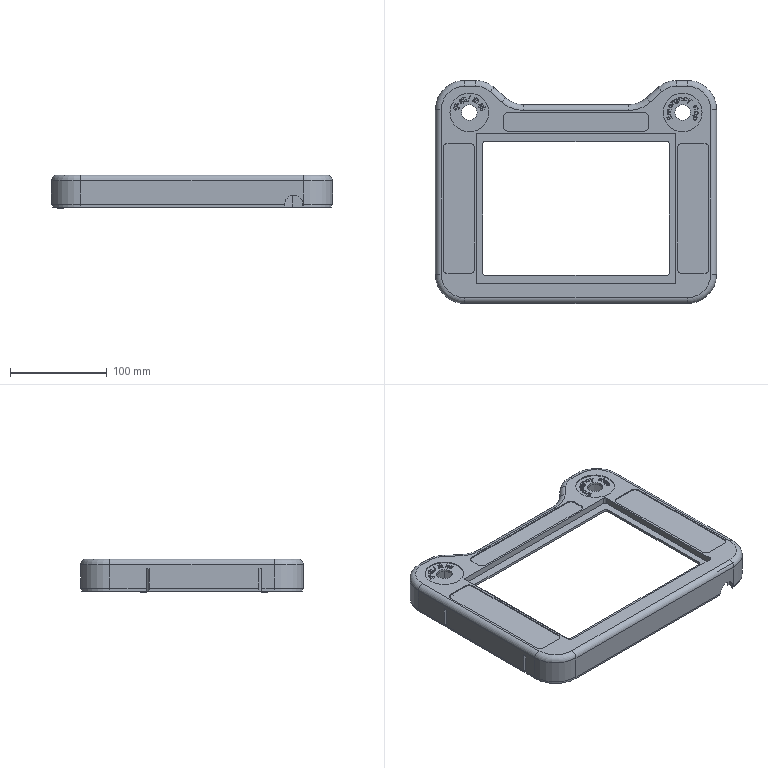Part | STEP file | 10B | 1 solid | 635 faces | box 290 x 230 x 35 mm | volume 178188 mm3 | plane 342 | cylinder 141 | spline 130 | torus 16 | cone 6 | commonest cylinder face diameters 2.6 x16 6 x16 15 x15 7 x12 10 x12 12 x12